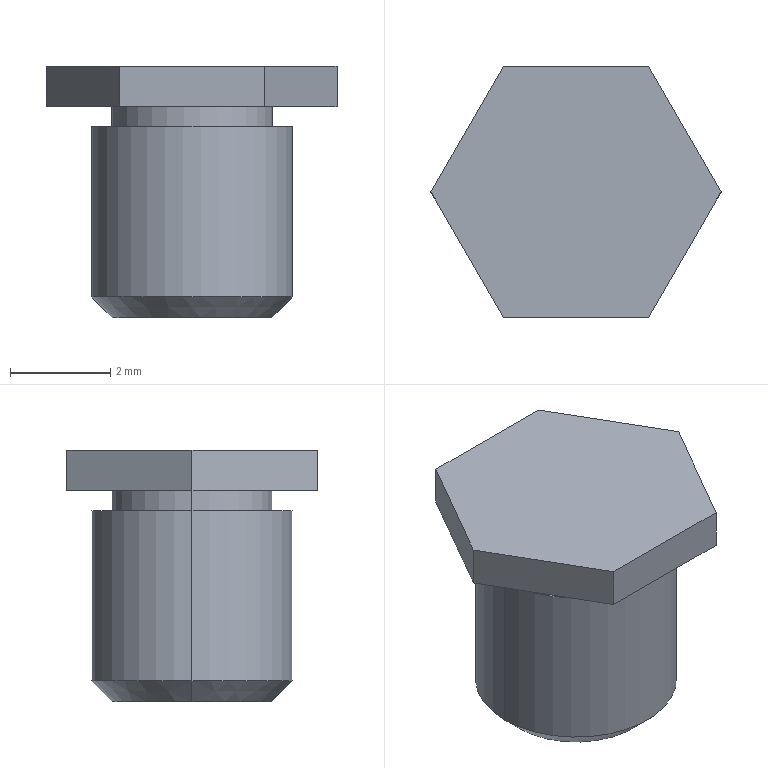Part | NX | features BREP 1 | 1 solid | 16 faces | box 5.774 x 5 x 5 mm | volume 67.305 mm3 | plane 10 | cylinder 4 | cone 2 | commonest cylinder face diameters 3.2 x2 4 x2
STEP:
#1=CARTESIAN_POINT('',(502.81,384.5,9.2));
#2=VERTEX_POINT('',#1);
#3=CARTESIAN_POINT('',(506.01,384.5,9.2));
#4=VERTEX_POINT('',#3);
#5=CARTESIAN_POINT('',(504.41,384.5,9.2));
#6=DIRECTION('',(0.,0.,-1.));
#7=DIRECTION('',(-1.,0.,0.));
#8=AXIS2_PLACEMENT_3D('',#5,#6,#7);
#9=CIRCLE('',#8,1.6);
#10=EDGE_CURVE('',#2,#4,#9,.T.);
#11=ORIENTED_EDGE('',*,*,#10,.T.);
#12=CARTESIAN_POINT('',(506.01,384.5,8.8));
#13=VERTEX_POINT('',#12);
#14=CARTESIAN_POINT('',(506.01,384.5,9.2));
#15=DIRECTION('',(0.,0.,-1.));
#16=VECTOR('',#15,1000.);
#17=LINE('',#14,#16);
#18=EDGE_CURVE('',#13,#4,#17,.F.);
#19=ORIENTED_EDGE('',*,*,#18,.F.);
#20=CARTESIAN_POINT('',(502.81,384.5,8.8));
#21=VERTEX_POINT('',#20);
#22=CARTESIAN_POINT('',(504.41,384.5,8.8));
#23=DIRECTION('',(0.,0.,1.));
#24=DIRECTION('',(-1.,0.,0.));
#25=AXIS2_PLACEMENT_3D('',#22,#23,#24);
#26=CIRCLE('',#25,1.6);
#27=EDGE_CURVE('',#13,#21,#26,.T.);
#28=ORIENTED_EDGE('',*,*,#27,.T.);
#29=CARTESIAN_POINT('',(502.81,384.5,9.2));
#30=DIRECTION('',(0.,0.,-1.));
#31=VECTOR('',#30,1000.);
#32=LINE('',#29,#31);
#33=EDGE_CURVE('',#21,#2,#32,.F.);
#34=ORIENTED_EDGE('',*,*,#33,.T.);
#35=EDGE_LOOP('',(#11,#19,#28,#34));
#36=FACE_BOUND('',#35,.T.);
#37=CARTESIAN_POINT('',(504.41,384.5,9.2));
#38=DIRECTION('',(0.,0.,-1.));
#39=DIRECTION('',(1.,0.,0.));
#40=AXIS2_PLACEMENT_3D('',#37,#38,#39);
#41=CYLINDRICAL_SURFACE('',#40,1.6);
#42=ADVANCED_FACE('',(#36),#41,.T.);
#43=CARTESIAN_POINT('',(506.41,384.5,5.41));
#44=VERTEX_POINT('',#43);
#45=CARTESIAN_POINT('',(502.41,384.5,5.41));
#46=VERTEX_POINT('',#45);
#47=CARTESIAN_POINT('',(504.41,384.5,5.41));
#48=DIRECTION('',(0.,0.,1.));
#49=DIRECTION('',(1.,0.,0.));
#50=AXIS2_PLACEMENT_3D('',#47,#48,#49);
#51=CIRCLE('',#50,2.);
#52=EDGE_CURVE('',#44,#46,#51,.T.);
#53=ORIENTED_EDGE('',*,*,#52,.T.);
#54=CARTESIAN_POINT('',(502.41,384.5,8.8));
#55=VERTEX_POINT('',#54);
#56=CARTESIAN_POINT('',(502.41,384.5,8.8));
#57=DIRECTION('',(0.,0.,1.));
#58=VECTOR('',#57,1000.);
#59=LINE('',#56,#58);
#60=EDGE_CURVE('',#46,#55,#59,.T.);
#61=ORIENTED_EDGE('',*,*,#60,.T.);
#62=CARTESIAN_POINT('',(506.41,384.5,8.8));
#63=VERTEX_POINT('',#62);
#64=CARTESIAN_POINT('',(504.41,384.5,8.8));
#65=DIRECTION('',(0.,0.,-1.));
#66=DIRECTION('',(1.,0.,0.));
#67=AXIS2_PLACEMENT_3D('',#64,#65,#66);
#68=CIRCLE('',#67,2.);
#69=EDGE_CURVE('',#55,#63,#68,.T.);
#70=ORIENTED_EDGE('',*,*,#69,.T.);
#71=CARTESIAN_POINT('',(506.41,384.5,8.8));
#72=DIRECTION('',(0.,0.,1.));
#73=VECTOR('',#72,1000.);
#74=LINE('',#71,#73);
#75=EDGE_CURVE('',#44,#63,#74,.T.);
#76=ORIENTED_EDGE('',*,*,#75,.F.);
#77=EDGE_LOOP('',(#53,#61,#70,#76));
#78=FACE_BOUND('',#77,.T.);
#79=CARTESIAN_POINT('',(504.41,384.5,8.8));
#80=DIRECTION('',(0.,0.,1.));
#81=DIRECTION('',(-1.,0.,0.));
#82=AXIS2_PLACEMENT_3D('',#79,#80,#81);
#83=CYLINDRICAL_SURFACE('',#82,2.);
#84=ADVANCED_FACE('',(#78),#83,.T.);
#85=CARTESIAN_POINT('',(506.,384.5,5.));
#86=VERTEX_POINT('',#85);
#87=CARTESIAN_POINT('',(502.82,384.5,5.));
#88=VERTEX_POINT('',#87);
#89=CARTESIAN_POINT('',(504.41,384.5,5.));
#90=DIRECTION('',(0.,0.,1.));
#91=DIRECTION('',(1.,0.,0.));
#92=AXIS2_PLACEMENT_3D('',#89,#90,#91);
#93=CIRCLE('',#92,1.59);
#94=EDGE_CURVE('',#86,#88,#93,.T.);
#95=ORIENTED_EDGE('',*,*,#94,.T.);
#96=CARTESIAN_POINT('',(502.41,384.5,5.41));
#97=DIRECTION('',(-0.7071,0.,0.7071));
#98=VECTOR('',#97,1000.);
#99=LINE('',#96,#98);
#100=EDGE_CURVE('',#88,#46,#99,.T.);
#101=ORIENTED_EDGE('',*,*,#100,.T.);
#102=ORIENTED_EDGE('',*,*,#52,.F.);
#103=CARTESIAN_POINT('',(506.41,384.5,5.41));
#104=DIRECTION('',(0.7071,0.,0.7071));
#105=VECTOR('',#104,1000.);
#106=LINE('',#103,#105);
#107=EDGE_CURVE('',#86,#44,#106,.T.);
#108=ORIENTED_EDGE('',*,*,#107,.F.);
#109=EDGE_LOOP('',(#95,#101,#102,#108));
#110=FACE_BOUND('',#109,.T.);
#111=CARTESIAN_POINT('',(504.41,384.5,5.41));
#112=DIRECTION('',(0.,0.,1.));
#113=DIRECTION('',(-1.,0.,0.));
#114=AXIS2_PLACEMENT_3D('',#111,#112,#113);
#115=CONICAL_SURFACE('',#114,2.,0.7854);
#116=ADVANCED_FACE('',(#110),#115,.T.);
#117=CARTESIAN_POINT('',(501.523,384.5,10.));
#118=VERTEX_POINT('',#117);
#119=CARTESIAN_POINT('',(502.967,382.,10.));
#120=VERTEX_POINT('',#119);
#121=CARTESIAN_POINT('',(501.523,384.5,10.));
#122=DIRECTION('',(0.5,-0.866,0.));
#123=VECTOR('',#122,1000.);
#124=LINE('',#121,#123);
#125=EDGE_CURVE('',#118,#120,#124,.T.);
#126=ORIENTED_EDGE('',*,*,#125,.T.);
#127=CARTESIAN_POINT('',(505.853,382.,10.));
#128=VERTEX_POINT('',#127);
#129=CARTESIAN_POINT('',(504.41,382.,10.));
#130=DIRECTION('',(1.,0.,0.));
#131=VECTOR('',#130,1000.);
#132=LINE('',#129,#131);
#133=EDGE_CURVE('',#120,#128,#132,.T.);
#134=ORIENTED_EDGE('',*,*,#133,.T.);
#135=CARTESIAN_POINT('',(507.297,384.5,10.));
#136=VERTEX_POINT('',#135);
#137=CARTESIAN_POINT('',(505.853,382.,10.));
#138=DIRECTION('',(0.5,0.866,0.));
#139=VECTOR('',#138,1000.);
#140=LINE('',#137,#139);
#141=EDGE_CURVE('',#128,#136,#140,.T.);
#142=ORIENTED_EDGE('',*,*,#141,.T.);
#143=CARTESIAN_POINT('',(505.853,387.,10.));
#144=VERTEX_POINT('',#143);
#145=CARTESIAN_POINT('',(507.297,384.5,10.));
#146=DIRECTION('',(-0.5,0.866,0.));
#147=VECTOR('',#146,1000.);
#148=LINE('',#145,#147);
#149=EDGE_CURVE('',#136,#144,#148,.T.);
#150=ORIENTED_EDGE('',*,*,#149,.T.);
#151=CARTESIAN_POINT('',(502.967,387.,10.));
#152=VERTEX_POINT('',#151);
#153=CARTESIAN_POINT('',(505.853,387.,10.));
#154=DIRECTION('',(-1.,0.00003829,0.));
#155=VECTOR('',#154,1000.);
#156=LINE('',#153,#155);
#157=EDGE_CURVE('',#144,#152,#156,.T.);
#158=ORIENTED_EDGE('',*,*,#157,.T.);
#159=CARTESIAN_POINT('',(502.967,387.,10.));
#160=DIRECTION('',(-0.5,-0.866,0.));
#161=VECTOR('',#160,1000.);
#162=LINE('',#159,#161);
#163=EDGE_CURVE('',#152,#118,#162,.T.);
#164=ORIENTED_EDGE('',*,*,#163,.T.);
#165=EDGE_LOOP('',(#126,#134,#142,#150,#158,#164));
#166=FACE_BOUND('',#165,.T.);
#167=CARTESIAN_POINT('',(504.41,384.5,10.));
#168=DIRECTION('',(0.,0.,1.));
#169=DIRECTION('',(-1.,0.,0.));
#170=AXIS2_PLACEMENT_3D('',#167,#168,#169);
#171=PLANE('',#170);
#172=ADVANCED_FACE('',(#166),#171,.T.);
#173=ORIENTED_EDGE('',*,*,#133,.F.);
#174=CARTESIAN_POINT('',(502.967,382.,9.2));
#175=VERTEX_POINT('',#174);
#176=CARTESIAN_POINT('',(502.967,382.,10.));
#177=DIRECTION('',(0.,0.,-1.));
#178=VECTOR('',#177,1000.);
#179=LINE('',#176,#178);
#180=EDGE_CURVE('',#120,#175,#179,.T.);
#181=ORIENTED_EDGE('',*,*,#180,.T.);
#182=CARTESIAN_POINT('',(505.853,382.,9.2));
#183=VERTEX_POINT('',#182);
#184=CARTESIAN_POINT('',(502.967,382.,9.2));
#185=DIRECTION('',(1.,0.,0.));
#186=VECTOR('',#185,1000.);
#187=LINE('',#184,#186);
#188=EDGE_CURVE('',#175,#183,#187,.T.);
#189=ORIENTED_EDGE('',*,*,#188,.T.);
#190=CARTESIAN_POINT('',(505.853,382.,10.));
#191=DIRECTION('',(0.,0.,1.));
#192=VECTOR('',#191,1000.);
#193=LINE('',#190,#192);
#194=EDGE_CURVE('',#183,#128,#193,.T.);
#195=ORIENTED_EDGE('',*,*,#194,.T.);
#196=EDGE_LOOP('',(#173,#181,#189,#195));
#197=FACE_BOUND('',#196,.T.);
#198=CARTESIAN_POINT('',(502.967,382.,10.));
#199=DIRECTION('',(0.,-1.,0.));
#200=DIRECTION('',(0.,0.,1.));
#201=AXIS2_PLACEMENT_3D('',#198,#199,#200);
#202=PLANE('',#201);
#203=ADVANCED_FACE('',(#197),#202,.T.);
#204=CARTESIAN_POINT('',(501.523,384.5,9.2));
#205=VERTEX_POINT('',#204);
#206=CARTESIAN_POINT('',(501.523,384.5,9.2));
#207=DIRECTION('',(0.5,-0.866,0.));
#208=VECTOR('',#207,1000.);
#209=LINE('',#206,#208);
#210=EDGE_CURVE('',#205,#175,#209,.T.);
#211=ORIENTED_EDGE('',*,*,#210,.T.);
#212=ORIENTED_EDGE('',*,*,#180,.F.);
#213=ORIENTED_EDGE('',*,*,#125,.F.);
#214=CARTESIAN_POINT('',(501.523,384.5,10.));
#215=DIRECTION('',(0.,0.,-1.));
#216=VECTOR('',#215,1000.);
#217=LINE('',#214,#216);
#218=EDGE_CURVE('',#118,#205,#217,.T.);
#219=ORIENTED_EDGE('',*,*,#218,.T.);
#220=EDGE_LOOP('',(#211,#212,#213,#219));
#221=FACE_BOUND('',#220,.T.);
#222=CARTESIAN_POINT('',(501.523,384.5,10.));
#223=DIRECTION('',(-0.866,-0.5,0.));
#224=DIRECTION('',(-0.5,0.866,0.));
#225=AXIS2_PLACEMENT_3D('',#222,#223,#224);
#226=PLANE('',#225);
#227=ADVANCED_FACE('',(#221),#226,.T.);
#228=ORIENTED_EDGE('',*,*,#163,.F.);
#229=CARTESIAN_POINT('',(502.967,387.,9.2));
#230=VERTEX_POINT('',#229);
#231=CARTESIAN_POINT('',(502.967,387.,10.));
#232=DIRECTION('',(0.,0.,-1.));
#233=VECTOR('',#232,1000.);
#234=LINE('',#231,#233);
#235=EDGE_CURVE('',#152,#230,#234,.T.);
#236=ORIENTED_EDGE('',*,*,#235,.T.);
#237=CARTESIAN_POINT('',(502.967,387.,9.2));
#238=DIRECTION('',(-0.5,-0.866,0.));
#239=VECTOR('',#238,1000.);
#240=LINE('',#237,#239);
#241=EDGE_CURVE('',#230,#205,#240,.T.);
#242=ORIENTED_EDGE('',*,*,#241,.T.);
#243=ORIENTED_EDGE('',*,*,#218,.F.);
#244=EDGE_LOOP('',(#228,#236,#242,#243));
#245=FACE_BOUND('',#244,.T.);
#246=CARTESIAN_POINT('',(502.967,387.,10.));
#247=DIRECTION('',(-0.866,0.5,0.));
#248=DIRECTION('',(0.5,0.866,0.));
#249=AXIS2_PLACEMENT_3D('',#246,#247,#248);
#250=PLANE('',#249);
#251=ADVANCED_FACE('',(#245),#250,.T.);
#252=ORIENTED_EDGE('',*,*,#157,.F.);
#253=CARTESIAN_POINT('',(505.853,387.,9.2));
#254=VERTEX_POINT('',#253);
#255=CARTESIAN_POINT('',(505.853,387.,9.2));
#256=DIRECTION('',(0.,0.,-1.));
#257=VECTOR('',#256,1000.);
#258=LINE('',#255,#257);
#259=EDGE_CURVE('',#144,#254,#258,.T.);
#260=ORIENTED_EDGE('',*,*,#259,.T.);
#261=CARTESIAN_POINT('',(504.452,387.,9.2));
#262=DIRECTION('',(-1.,0.00003827,0.));
#263=VECTOR('',#262,1000.);
#264=LINE('',#261,#263);
#265=EDGE_CURVE('',#254,#230,#264,.T.);
#266=ORIENTED_EDGE('',*,*,#265,.T.);
#267=ORIENTED_EDGE('',*,*,#235,.F.);
#268=EDGE_LOOP('',(#252,#260,#266,#267));
#269=FACE_BOUND('',#268,.T.);
#270=CARTESIAN_POINT('',(504.452,387.,9.2));
#271=DIRECTION('',(0.00003827,1.,0.));
#272=DIRECTION('',(1.,-0.00003827,0.));
#273=AXIS2_PLACEMENT_3D('',#270,#271,#272);
#274=PLANE('',#273);
#275=ADVANCED_FACE('',(#269),#274,.T.);
#276=ORIENTED_EDGE('',*,*,#149,.F.);
#277=CARTESIAN_POINT('',(507.297,384.5,9.2));
#278=VERTEX_POINT('',#277);
#279=CARTESIAN_POINT('',(507.297,384.5,10.));
#280=DIRECTION('',(0.,0.,-1.));
#281=VECTOR('',#280,1000.);
#282=LINE('',#279,#281);
#283=EDGE_CURVE('',#136,#278,#282,.T.);
#284=ORIENTED_EDGE('',*,*,#283,.T.);
#285=CARTESIAN_POINT('',(507.297,384.5,9.2));
#286=DIRECTION('',(-0.5,0.866,0.));
#287=VECTOR('',#286,1000.);
#288=LINE('',#285,#287);
#289=EDGE_CURVE('',#278,#254,#288,.T.);
#290=ORIENTED_EDGE('',*,*,#289,.T.);
#291=ORIENTED_EDGE('',*,*,#259,.F.);
#292=EDGE_LOOP('',(#276,#284,#290,#291));
#293=FACE_BOUND('',#292,.T.);
#294=CARTESIAN_POINT('',(507.297,384.5,10.));
#295=DIRECTION('',(0.866,0.5,0.));
#296=DIRECTION('',(0.5,-0.866,0.));
#297=AXIS2_PLACEMENT_3D('',#294,#295,#296);
#298=PLANE('',#297);
#299=ADVANCED_FACE('',(#293),#298,.T.);
#300=CARTESIAN_POINT('',(505.853,382.,9.2));
#301=DIRECTION('',(0.5,0.866,0.));
#302=VECTOR('',#301,1000.);
#303=LINE('',#300,#302);
#304=EDGE_CURVE('',#183,#278,#303,.T.);
#305=ORIENTED_EDGE('',*,*,#304,.T.);
#306=ORIENTED_EDGE('',*,*,#283,.F.);
#307=ORIENTED_EDGE('',*,*,#141,.F.);
#308=ORIENTED_EDGE('',*,*,#194,.F.);
#309=EDGE_LOOP('',(#305,#306,#307,#308));
#310=FACE_BOUND('',#309,.T.);
#311=CARTESIAN_POINT('',(505.853,382.,10.));
#312=DIRECTION('',(0.866,-0.5,0.));
#313=DIRECTION('',(-0.5,-0.866,0.));
#314=AXIS2_PLACEMENT_3D('',#311,#312,#313);
#315=PLANE('',#314);
#316=ADVANCED_FACE('',(#310),#315,.T.);
#317=ORIENTED_EDGE('',*,*,#265,.F.);
#318=ORIENTED_EDGE('',*,*,#289,.F.);
#319=ORIENTED_EDGE('',*,*,#304,.F.);
#320=ORIENTED_EDGE('',*,*,#188,.F.);
#321=ORIENTED_EDGE('',*,*,#210,.F.);
#322=ORIENTED_EDGE('',*,*,#241,.F.);
#323=EDGE_LOOP('',(#317,#318,#319,#320,#321,#322));
#324=FACE_BOUND('',#323,.T.);
#325=ORIENTED_EDGE('',*,*,#10,.F.);
#326=CARTESIAN_POINT('',(504.41,384.5,9.2));
#327=DIRECTION('',(0.,0.,-1.));
#328=DIRECTION('',(-1.,0.,0.));
#329=AXIS2_PLACEMENT_3D('',#326,#327,#328);
#330=CIRCLE('',#329,1.6);
#331=EDGE_CURVE('',#4,#2,#330,.T.);
#332=ORIENTED_EDGE('',*,*,#331,.F.);
#333=EDGE_LOOP('',(#325,#332));
#334=FACE_BOUND('',#333,.T.);
#335=CARTESIAN_POINT('',(504.41,384.5,9.2));
#336=DIRECTION('',(0.,0.,1.));
#337=DIRECTION('',(-1.,0.,0.));
#338=AXIS2_PLACEMENT_3D('',#335,#336,#337);
#339=PLANE('',#338);
#340=ADVANCED_FACE('',(#324,#334),#339,.F.);
#341=ORIENTED_EDGE('',*,*,#18,.T.);
#342=ORIENTED_EDGE('',*,*,#331,.T.);
#343=ORIENTED_EDGE('',*,*,#33,.F.);
#344=CARTESIAN_POINT('',(504.41,384.5,8.8));
#345=DIRECTION('',(0.,0.,1.));
#346=DIRECTION('',(-1.,0.,0.));
#347=AXIS2_PLACEMENT_3D('',#344,#345,#346);
#348=CIRCLE('',#347,1.6);
#349=EDGE_CURVE('',#21,#13,#348,.T.);
#350=ORIENTED_EDGE('',*,*,#349,.T.);
#351=EDGE_LOOP('',(#341,#342,#343,#350));
#352=FACE_BOUND('',#351,.T.);
#353=CARTESIAN_POINT('',(504.41,384.5,9.2));
#354=DIRECTION('',(0.,0.,-1.));
#355=DIRECTION('',(1.,0.,0.));
#356=AXIS2_PLACEMENT_3D('',#353,#354,#355);
#357=CYLINDRICAL_SURFACE('',#356,1.6);
#358=ADVANCED_FACE('',(#352),#357,.T.);
#359=CARTESIAN_POINT('',(504.41,384.5,8.8));
#360=DIRECTION('',(0.,0.,-1.));
#361=DIRECTION('',(1.,0.,0.));
#362=AXIS2_PLACEMENT_3D('',#359,#360,#361);
#363=CIRCLE('',#362,2.);
#364=EDGE_CURVE('',#63,#55,#363,.T.);
#365=ORIENTED_EDGE('',*,*,#364,.F.);
#366=ORIENTED_EDGE('',*,*,#69,.F.);
#367=EDGE_LOOP('',(#365,#366));
#368=FACE_BOUND('',#367,.T.);
#369=ORIENTED_EDGE('',*,*,#349,.F.);
#370=ORIENTED_EDGE('',*,*,#27,.F.);
#371=EDGE_LOOP('',(#369,#370));
#372=FACE_BOUND('',#371,.T.);
#373=CARTESIAN_POINT('',(504.41,384.5,8.8));
#374=DIRECTION('',(0.,0.,-1.));
#375=DIRECTION('',(1.,0.,0.));
#376=AXIS2_PLACEMENT_3D('',#373,#374,#375);
#377=PLANE('',#376);
#378=ADVANCED_FACE('',(#368,#372),#377,.F.);
#379=ORIENTED_EDGE('',*,*,#60,.F.);
#380=CARTESIAN_POINT('',(504.41,384.5,5.41));
#381=DIRECTION('',(0.,0.,1.));
#382=DIRECTION('',(1.,0.,0.));
#383=AXIS2_PLACEMENT_3D('',#380,#381,#382);
#384=CIRCLE('',#383,2.);
#385=EDGE_CURVE('',#46,#44,#384,.T.);
#386=ORIENTED_EDGE('',*,*,#385,.T.);
#387=ORIENTED_EDGE('',*,*,#75,.T.);
#388=ORIENTED_EDGE('',*,*,#364,.T.);
#389=EDGE_LOOP('',(#379,#386,#387,#388));
#390=FACE_BOUND('',#389,.T.);
#391=CARTESIAN_POINT('',(504.41,384.5,8.8));
#392=DIRECTION('',(0.,0.,1.));
#393=DIRECTION('',(-1.,0.,0.));
#394=AXIS2_PLACEMENT_3D('',#391,#392,#393);
#395=CYLINDRICAL_SURFACE('',#394,2.);
#396=ADVANCED_FACE('',(#390),#395,.T.);
#397=ORIENTED_EDGE('',*,*,#100,.F.);
#398=CARTESIAN_POINT('',(504.41,384.5,5.));
#399=DIRECTION('',(0.,0.,1.));
#400=DIRECTION('',(1.,0.,0.));
#401=AXIS2_PLACEMENT_3D('',#398,#399,#400);
#402=CIRCLE('',#401,1.59);
#403=EDGE_CURVE('',#88,#86,#402,.T.);
#404=ORIENTED_EDGE('',*,*,#403,.T.);
#405=ORIENTED_EDGE('',*,*,#107,.T.);
#406=ORIENTED_EDGE('',*,*,#385,.F.);
#407=EDGE_LOOP('',(#397,#404,#405,#406));
#408=FACE_BOUND('',#407,.T.);
#409=CARTESIAN_POINT('',(504.41,384.5,5.41));
#410=DIRECTION('',(0.,0.,1.));
#411=DIRECTION('',(-1.,0.,0.));
#412=AXIS2_PLACEMENT_3D('',#409,#410,#411);
#413=CONICAL_SURFACE('',#412,2.,0.7854);
#414=ADVANCED_FACE('',(#408),#413,.T.);
#415=ORIENTED_EDGE('',*,*,#94,.F.);
#416=ORIENTED_EDGE('',*,*,#403,.F.);
#417=EDGE_LOOP('',(#415,#416));
#418=FACE_BOUND('',#417,.T.);
#419=CARTESIAN_POINT('',(504.41,384.5,5.));
#420=DIRECTION('',(0.,0.,-1.));
#421=DIRECTION('',(1.,0.,0.));
#422=AXIS2_PLACEMENT_3D('',#419,#420,#421);
#423=PLANE('',#422);
#424=ADVANCED_FACE('',(#418),#423,.T.);
#425=CLOSED_SHELL('',(#42,#84,#116,#172,#203,#227,#251,#275,#299,#316,#340,#358,#378,#396,#414,#424));
#426=MANIFOLD_SOLID_BREP('',#425);
#427=(LENGTH_UNIT()NAMED_UNIT(*)SI_UNIT(.MILLI.,.METRE.));
#428=UNCERTAINTY_MEASURE_WITH_UNIT(LENGTH_MEASURE(0.00001),#427,'','');
#429=(NAMED_UNIT(*)PLANE_ANGLE_UNIT()SI_UNIT($,.RADIAN.));
#430=(NAMED_UNIT(*)SI_UNIT($,.STERADIAN.)SOLID_ANGLE_UNIT());
#431=(GEOMETRIC_REPRESENTATION_CONTEXT(3)GLOBAL_UNCERTAINTY_ASSIGNED_CONTEXT((#428))GLOBAL_UNIT_ASSIGNED_CONTEXT((#427,#429,#430))REPRESENTATION_CONTEXT('',''));
#432=ADVANCED_BREP_SHAPE_REPRESENTATION('',(#426),#431);